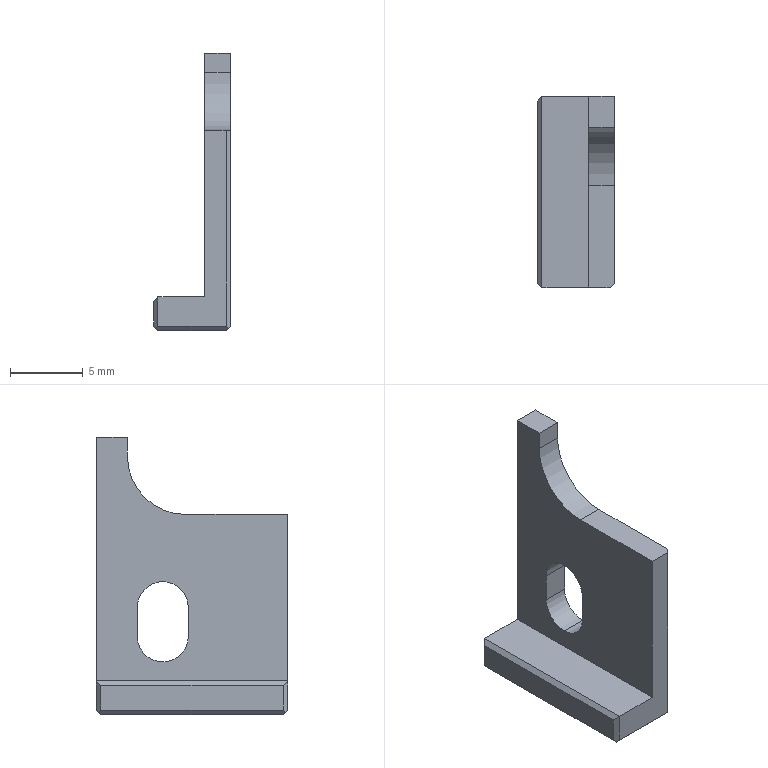Part | NX | 1 solid | 24 faces | box 5.273 x 13.1 x 19 mm | volume 417.678 mm3 | plane 20 | cylinder 4 | commonest cylinder face diameters 3.5 x3 8 x1
STEP:
#1=CARTESIAN_POINT('',(1996.107,151.5,-109.));
#2=VERTEX_POINT('',#1);
#3=CARTESIAN_POINT('',(1997.581,151.5,-109.));
#4=VERTEX_POINT('',#3);
#5=CARTESIAN_POINT('',(1996.994,151.5,-109.));
#6=DIRECTION('',(1.,0.,0.));
#7=VECTOR('',#6,1000.);
#8=LINE('',#5,#7);
#9=EDGE_CURVE('',#2,#4,#8,.T.);
#10=ORIENTED_EDGE('',*,*,#9,.F.);
#11=CARTESIAN_POINT('',(1996.107,151.5,-120.418));
#12=VERTEX_POINT('',#11);
#13=CARTESIAN_POINT('',(1996.107,151.5,-103.718));
#14=DIRECTION('',(0.,0.,-1.));
#15=VECTOR('',#14,1000.);
#16=LINE('',#13,#15);
#17=EDGE_CURVE('',#2,#12,#16,.T.);
#18=ORIENTED_EDGE('',*,*,#17,.T.);
#19=CARTESIAN_POINT('',(1992.907,151.5,-120.418));
#20=VERTEX_POINT('',#19);
#21=CARTESIAN_POINT('',(1996.107,151.5,-120.418));
#22=DIRECTION('',(-1.,0.,0.));
#23=VECTOR('',#22,1000.);
#24=LINE('',#21,#23);
#25=EDGE_CURVE('',#12,#20,#24,.T.);
#26=ORIENTED_EDGE('',*,*,#25,.T.);
#27=CARTESIAN_POINT('',(1992.907,151.5,-122.418));
#28=VERTEX_POINT('',#27);
#29=CARTESIAN_POINT('',(1992.907,151.5,-121.568));
#30=DIRECTION('',(0.,0.,-1.));
#31=VECTOR('',#30,1000.);
#32=LINE('',#29,#31);
#33=EDGE_CURVE('',#20,#28,#32,.T.);
#34=ORIENTED_EDGE('',*,*,#33,.T.);
#35=CARTESIAN_POINT('',(1997.581,151.5,-122.418));
#36=VERTEX_POINT('',#35);
#37=CARTESIAN_POINT('',(1995.244,151.5,-122.418));
#38=DIRECTION('',(-1.,0.,0.));
#39=VECTOR('',#38,1000.);
#40=LINE('',#37,#39);
#41=EDGE_CURVE('',#36,#28,#40,.T.);
#42=ORIENTED_EDGE('',*,*,#41,.F.);
#43=CARTESIAN_POINT('',(1997.581,151.5,-103.718));
#44=DIRECTION('',(0.,0.,-1.));
#45=VECTOR('',#44,1000.);
#46=LINE('',#43,#45);
#47=EDGE_CURVE('',#4,#36,#46,.T.);
#48=ORIENTED_EDGE('',*,*,#47,.F.);
#49=EDGE_LOOP('',(#10,#18,#26,#34,#42,#48));
#50=FACE_BOUND('',#49,.T.);
#51=CARTESIAN_POINT('',(1997.881,151.5,-103.718));
#52=DIRECTION('',(0.,1.,0.));
#53=DIRECTION('',(1.,0.,0.));
#54=AXIS2_PLACEMENT_3D('',#51,#52,#53);
#55=PLANE('',#54);
#56=ADVANCED_FACE('',(#50),#55,.F.);
#57=CARTESIAN_POINT('',(1997.881,151.8,-109.));
#58=VERTEX_POINT('',#57);
#59=CARTESIAN_POINT('',(1997.881,151.8,-122.418));
#60=VERTEX_POINT('',#59);
#61=CARTESIAN_POINT('',(1997.881,151.8,-115.709));
#62=DIRECTION('',(0.,0.,-1.));
#63=VECTOR('',#62,1000.);
#64=LINE('',#61,#63);
#65=EDGE_CURVE('',#58,#60,#64,.T.);
#66=ORIENTED_EDGE('',*,*,#65,.T.);
#67=CARTESIAN_POINT('',(1997.881,164.6,-122.418));
#68=VERTEX_POINT('',#67);
#69=CARTESIAN_POINT('',(1997.881,158.05,-122.418));
#70=DIRECTION('',(0.,1.,0.));
#71=VECTOR('',#70,1000.);
#72=LINE('',#69,#71);
#73=EDGE_CURVE('',#60,#68,#72,.T.);
#74=ORIENTED_EDGE('',*,*,#73,.T.);
#75=CARTESIAN_POINT('',(1997.881,164.6,-103.718));
#76=VERTEX_POINT('',#75);
#77=CARTESIAN_POINT('',(1997.881,164.6,-103.718));
#78=DIRECTION('',(0.,0.,-1.));
#79=VECTOR('',#78,1000.);
#80=LINE('',#77,#79);
#81=EDGE_CURVE('',#76,#68,#80,.T.);
#82=ORIENTED_EDGE('',*,*,#81,.F.);
#83=CARTESIAN_POINT('',(1997.881,162.476,-103.718));
#84=VERTEX_POINT('',#83);
#85=CARTESIAN_POINT('',(1997.881,155.5,-103.718));
#86=DIRECTION('',(0.,1.,0.));
#87=VECTOR('',#86,1000.);
#88=LINE('',#85,#87);
#89=EDGE_CURVE('',#84,#76,#88,.T.);
#90=ORIENTED_EDGE('',*,*,#89,.F.);
#91=CARTESIAN_POINT('',(1997.881,162.476,-105.));
#92=VERTEX_POINT('',#91);
#93=CARTESIAN_POINT('',(1997.881,162.476,-103.718));
#94=DIRECTION('',(0.,0.,1.));
#95=VECTOR('',#94,1000.);
#96=LINE('',#93,#95);
#97=EDGE_CURVE('',#92,#84,#96,.T.);
#98=ORIENTED_EDGE('',*,*,#97,.F.);
#99=CARTESIAN_POINT('',(1997.881,158.476,-109.));
#100=VERTEX_POINT('',#99);
#101=CARTESIAN_POINT('',(1997.881,158.476,-105.));
#102=DIRECTION('',(1.,0.,0.));
#103=DIRECTION('',(0.,-1.,0.));
#104=AXIS2_PLACEMENT_3D('',#101,#102,#103);
#105=CIRCLE('',#104,4.);
#106=EDGE_CURVE('',#100,#92,#105,.T.);
#107=ORIENTED_EDGE('',*,*,#106,.F.);
#108=CARTESIAN_POINT('',(1997.881,163.538,-109.));
#109=DIRECTION('',(0.,1.,0.));
#110=VECTOR('',#109,1000.);
#111=LINE('',#108,#110);
#112=EDGE_CURVE('',#58,#100,#111,.T.);
#113=ORIENTED_EDGE('',*,*,#112,.F.);
#114=EDGE_LOOP('',(#66,#74,#82,#90,#98,#107,#113));
#115=FACE_BOUND('',#114,.T.);
#116=CARTESIAN_POINT('',(1997.881,158.3,-117.359));
#117=VERTEX_POINT('',#116);
#118=CARTESIAN_POINT('',(1997.881,158.3,-115.359));
#119=VERTEX_POINT('',#118);
#120=CARTESIAN_POINT('',(1997.881,158.3,-103.718));
#121=DIRECTION('',(0.,0.,1.));
#122=VECTOR('',#121,1000.);
#123=LINE('',#120,#122);
#124=EDGE_CURVE('',#117,#119,#123,.T.);
#125=ORIENTED_EDGE('',*,*,#124,.T.);
#126=CARTESIAN_POINT('',(1997.881,161.8,-115.359));
#127=VERTEX_POINT('',#126);
#128=CARTESIAN_POINT('',(1997.881,160.05,-115.359));
#129=DIRECTION('',(1.,0.,0.));
#130=DIRECTION('',(0.,0.,-1.));
#131=AXIS2_PLACEMENT_3D('',#128,#129,#130);
#132=CIRCLE('',#131,1.75);
#133=EDGE_CURVE('',#127,#119,#132,.T.);
#134=ORIENTED_EDGE('',*,*,#133,.F.);
#135=CARTESIAN_POINT('',(1997.881,161.8,-117.359));
#136=VERTEX_POINT('',#135);
#137=CARTESIAN_POINT('',(1997.881,161.8,-103.718));
#138=DIRECTION('',(0.,0.,-1.));
#139=VECTOR('',#138,1000.);
#140=LINE('',#137,#139);
#141=EDGE_CURVE('',#127,#136,#140,.T.);
#142=ORIENTED_EDGE('',*,*,#141,.T.);
#143=CARTESIAN_POINT('',(1997.881,160.05,-119.109));
#144=VERTEX_POINT('',#143);
#145=CARTESIAN_POINT('',(1997.881,160.05,-117.359));
#146=DIRECTION('',(1.,0.,0.));
#147=DIRECTION('',(0.,0.,-1.));
#148=AXIS2_PLACEMENT_3D('',#145,#146,#147);
#149=CIRCLE('',#148,1.75);
#150=EDGE_CURVE('',#144,#136,#149,.T.);
#151=ORIENTED_EDGE('',*,*,#150,.F.);
#152=CARTESIAN_POINT('',(1997.881,160.05,-117.359));
#153=DIRECTION('',(1.,0.,0.));
#154=DIRECTION('',(0.,0.,-1.));
#155=AXIS2_PLACEMENT_3D('',#152,#153,#154);
#156=CIRCLE('',#155,1.75);
#157=EDGE_CURVE('',#117,#144,#156,.T.);
#158=ORIENTED_EDGE('',*,*,#157,.F.);
#159=EDGE_LOOP('',(#125,#134,#142,#151,#158));
#160=FACE_BOUND('',#159,.T.);
#161=CARTESIAN_POINT('',(1997.881,164.6,-103.718));
#162=DIRECTION('',(-1.,0.,0.));
#163=DIRECTION('',(0.,0.,1.));
#164=AXIS2_PLACEMENT_3D('',#161,#162,#163);
#165=PLANE('',#164);
#166=ADVANCED_FACE('',(#115,#160),#165,.F.);
#167=CARTESIAN_POINT('',(1996.107,158.476,-109.));
#168=VERTEX_POINT('',#167);
#169=CARTESIAN_POINT('',(1996.107,163.538,-109.));
#170=DIRECTION('',(0.,-1.,0.));
#171=VECTOR('',#170,1000.);
#172=LINE('',#169,#171);
#173=EDGE_CURVE('',#168,#2,#172,.T.);
#174=ORIENTED_EDGE('',*,*,#173,.F.);
#175=CARTESIAN_POINT('',(1996.107,162.476,-105.));
#176=VERTEX_POINT('',#175);
#177=CARTESIAN_POINT('',(1996.107,158.476,-105.));
#178=DIRECTION('',(1.,0.,0.));
#179=DIRECTION('',(0.,-1.,0.));
#180=AXIS2_PLACEMENT_3D('',#177,#178,#179);
#181=CIRCLE('',#180,4.);
#182=EDGE_CURVE('',#168,#176,#181,.T.);
#183=ORIENTED_EDGE('',*,*,#182,.T.);
#184=CARTESIAN_POINT('',(1996.107,162.476,-103.718));
#185=VERTEX_POINT('',#184);
#186=CARTESIAN_POINT('',(1996.107,162.476,-103.718));
#187=DIRECTION('',(0.,0.,-1.));
#188=VECTOR('',#187,1000.);
#189=LINE('',#186,#188);
#190=EDGE_CURVE('',#185,#176,#189,.T.);
#191=ORIENTED_EDGE('',*,*,#190,.F.);
#192=CARTESIAN_POINT('',(1996.107,164.6,-103.718));
#193=VERTEX_POINT('',#192);
#194=CARTESIAN_POINT('',(1996.107,164.6,-103.718));
#195=DIRECTION('',(0.,-1.,0.));
#196=VECTOR('',#195,1000.);
#197=LINE('',#194,#196);
#198=EDGE_CURVE('',#193,#185,#197,.T.);
#199=ORIENTED_EDGE('',*,*,#198,.F.);
#200=CARTESIAN_POINT('',(1996.107,164.6,-120.418));
#201=VERTEX_POINT('',#200);
#202=CARTESIAN_POINT('',(1996.107,164.6,-103.718));
#203=DIRECTION('',(0.,0.,-1.));
#204=VECTOR('',#203,1000.);
#205=LINE('',#202,#204);
#206=EDGE_CURVE('',#193,#201,#205,.T.);
#207=ORIENTED_EDGE('',*,*,#206,.T.);
#208=CARTESIAN_POINT('',(1996.107,163.538,-120.418));
#209=DIRECTION('',(0.,-1.,0.));
#210=VECTOR('',#209,1000.);
#211=LINE('',#208,#210);
#212=EDGE_CURVE('',#201,#12,#211,.T.);
#213=ORIENTED_EDGE('',*,*,#212,.T.);
#214=ORIENTED_EDGE('',*,*,#17,.F.);
#215=EDGE_LOOP('',(#174,#183,#191,#199,#207,#213,#214));
#216=FACE_BOUND('',#215,.T.);
#217=CARTESIAN_POINT('',(1996.107,158.3,-115.359));
#218=VERTEX_POINT('',#217);
#219=CARTESIAN_POINT('',(1996.107,158.3,-117.359));
#220=VERTEX_POINT('',#219);
#221=CARTESIAN_POINT('',(1996.107,158.3,-103.718));
#222=DIRECTION('',(0.,0.,-1.));
#223=VECTOR('',#222,1000.);
#224=LINE('',#221,#223);
#225=EDGE_CURVE('',#218,#220,#224,.T.);
#226=ORIENTED_EDGE('',*,*,#225,.T.);
#227=CARTESIAN_POINT('',(1996.107,160.05,-119.109));
#228=VERTEX_POINT('',#227);
#229=CARTESIAN_POINT('',(1996.107,160.05,-117.359));
#230=DIRECTION('',(1.,0.,0.));
#231=DIRECTION('',(0.,0.,-1.));
#232=AXIS2_PLACEMENT_3D('',#229,#230,#231);
#233=CIRCLE('',#232,1.75);
#234=EDGE_CURVE('',#220,#228,#233,.T.);
#235=ORIENTED_EDGE('',*,*,#234,.T.);
#236=CARTESIAN_POINT('',(1996.107,161.8,-117.359));
#237=VERTEX_POINT('',#236);
#238=CARTESIAN_POINT('',(1996.107,160.05,-117.359));
#239=DIRECTION('',(1.,0.,0.));
#240=DIRECTION('',(0.,0.,-1.));
#241=AXIS2_PLACEMENT_3D('',#238,#239,#240);
#242=CIRCLE('',#241,1.75);
#243=EDGE_CURVE('',#228,#237,#242,.T.);
#244=ORIENTED_EDGE('',*,*,#243,.T.);
#245=CARTESIAN_POINT('',(1996.107,161.8,-115.359));
#246=VERTEX_POINT('',#245);
#247=CARTESIAN_POINT('',(1996.107,161.8,-103.718));
#248=DIRECTION('',(0.,0.,1.));
#249=VECTOR('',#248,1000.);
#250=LINE('',#247,#249);
#251=EDGE_CURVE('',#237,#246,#250,.T.);
#252=ORIENTED_EDGE('',*,*,#251,.T.);
#253=CARTESIAN_POINT('',(1996.107,160.05,-115.359));
#254=DIRECTION('',(1.,0.,0.));
#255=DIRECTION('',(0.,0.,-1.));
#256=AXIS2_PLACEMENT_3D('',#253,#254,#255);
#257=CIRCLE('',#256,1.75);
#258=EDGE_CURVE('',#246,#218,#257,.T.);
#259=ORIENTED_EDGE('',*,*,#258,.T.);
#260=EDGE_LOOP('',(#226,#235,#244,#252,#259));
#261=FACE_BOUND('',#260,.T.);
#262=CARTESIAN_POINT('',(1996.107,155.5,-103.718));
#263=DIRECTION('',(1.,0.,0.));
#264=DIRECTION('',(0.,1.,0.));
#265=AXIS2_PLACEMENT_3D('',#262,#263,#264);
#266=PLANE('',#265);
#267=ADVANCED_FACE('',(#216,#261),#266,.F.);
#268=CARTESIAN_POINT('',(1992.907,164.6,-122.418));
#269=VERTEX_POINT('',#268);
#270=CARTESIAN_POINT('',(1995.244,164.6,-122.418));
#271=DIRECTION('',(1.,0.,0.));
#272=VECTOR('',#271,1000.);
#273=LINE('',#270,#272);
#274=EDGE_CURVE('',#269,#68,#273,.T.);
#275=ORIENTED_EDGE('',*,*,#274,.F.);
#276=CARTESIAN_POINT('',(1992.907,164.6,-120.418));
#277=VERTEX_POINT('',#276);
#278=CARTESIAN_POINT('',(1992.907,164.6,-121.568));
#279=DIRECTION('',(0.,0.,1.));
#280=VECTOR('',#279,1000.);
#281=LINE('',#278,#280);
#282=EDGE_CURVE('',#269,#277,#281,.T.);
#283=ORIENTED_EDGE('',*,*,#282,.T.);
#284=CARTESIAN_POINT('',(1996.107,164.6,-120.418));
#285=DIRECTION('',(-1.,0.,0.));
#286=VECTOR('',#285,1000.);
#287=LINE('',#284,#286);
#288=EDGE_CURVE('',#201,#277,#287,.T.);
#289=ORIENTED_EDGE('',*,*,#288,.F.);
#290=ORIENTED_EDGE('',*,*,#206,.F.);
#291=CARTESIAN_POINT('',(2001.481,164.6,-103.718));
#292=DIRECTION('',(-1.,0.,0.));
#293=VECTOR('',#292,1000.);
#294=LINE('',#291,#293);
#295=EDGE_CURVE('',#76,#193,#294,.T.);
#296=ORIENTED_EDGE('',*,*,#295,.F.);
#297=ORIENTED_EDGE('',*,*,#81,.T.);
#298=EDGE_LOOP('',(#275,#283,#289,#290,#296,#297));
#299=FACE_BOUND('',#298,.T.);
#300=CARTESIAN_POINT('',(1996.107,164.6,-103.718));
#301=DIRECTION('',(0.,-1.,0.));
#302=DIRECTION('',(0.,0.,-1.));
#303=AXIS2_PLACEMENT_3D('',#300,#301,#302);
#304=PLANE('',#303);
#305=ADVANCED_FACE('',(#299),#304,.F.);
#306=CARTESIAN_POINT('',(1993.73,160.05,-119.109));
#307=DIRECTION('',(1.,0.,0.));
#308=VECTOR('',#307,1000.);
#309=LINE('',#306,#308);
#310=EDGE_CURVE('',#228,#144,#309,.T.);
#311=ORIENTED_EDGE('',*,*,#310,.F.);
#312=ORIENTED_EDGE('',*,*,#234,.F.);
#313=CARTESIAN_POINT('',(1993.73,158.3,-117.359));
#314=DIRECTION('',(1.,0.,0.));
#315=VECTOR('',#314,1000.);
#316=LINE('',#313,#315);
#317=EDGE_CURVE('',#220,#117,#316,.T.);
#318=ORIENTED_EDGE('',*,*,#317,.T.);
#319=ORIENTED_EDGE('',*,*,#157,.T.);
#320=EDGE_LOOP('',(#311,#312,#318,#319));
#321=FACE_BOUND('',#320,.T.);
#322=CARTESIAN_POINT('',(1993.73,160.05,-117.359));
#323=DIRECTION('',(1.,0.,0.));
#324=DIRECTION('',(0.,0.,-1.));
#325=AXIS2_PLACEMENT_3D('',#322,#323,#324);
#326=CYLINDRICAL_SURFACE('',#325,1.75);
#327=ADVANCED_FACE('',(#321),#326,.F.);
#328=ORIENTED_EDGE('',*,*,#251,.F.);
#329=CARTESIAN_POINT('',(1993.73,161.8,-117.359));
#330=DIRECTION('',(1.,0.,0.));
#331=VECTOR('',#330,1000.);
#332=LINE('',#329,#331);
#333=EDGE_CURVE('',#237,#136,#332,.T.);
#334=ORIENTED_EDGE('',*,*,#333,.T.);
#335=ORIENTED_EDGE('',*,*,#141,.F.);
#336=CARTESIAN_POINT('',(1993.73,161.8,-115.359));
#337=DIRECTION('',(1.,0.,0.));
#338=VECTOR('',#337,1000.);
#339=LINE('',#336,#338);
#340=EDGE_CURVE('',#246,#127,#339,.T.);
#341=ORIENTED_EDGE('',*,*,#340,.F.);
#342=EDGE_LOOP('',(#328,#334,#335,#341));
#343=FACE_BOUND('',#342,.T.);
#344=CARTESIAN_POINT('',(1993.73,161.8,-115.359));
#345=DIRECTION('',(0.,1.,0.));
#346=DIRECTION('',(1.,0.,0.));
#347=AXIS2_PLACEMENT_3D('',#344,#345,#346);
#348=PLANE('',#347);
#349=ADVANCED_FACE('',(#343),#348,.F.);
#350=ORIENTED_EDGE('',*,*,#258,.F.);
#351=ORIENTED_EDGE('',*,*,#340,.T.);
#352=ORIENTED_EDGE('',*,*,#133,.T.);
#353=CARTESIAN_POINT('',(1993.73,158.3,-115.359));
#354=DIRECTION('',(1.,0.,0.));
#355=VECTOR('',#354,1000.);
#356=LINE('',#353,#355);
#357=EDGE_CURVE('',#218,#119,#356,.T.);
#358=ORIENTED_EDGE('',*,*,#357,.F.);
#359=EDGE_LOOP('',(#350,#351,#352,#358));
#360=FACE_BOUND('',#359,.T.);
#361=CARTESIAN_POINT('',(1993.73,160.05,-115.359));
#362=DIRECTION('',(1.,0.,0.));
#363=DIRECTION('',(0.,0.,-1.));
#364=AXIS2_PLACEMENT_3D('',#361,#362,#363);
#365=CYLINDRICAL_SURFACE('',#364,1.75);
#366=ADVANCED_FACE('',(#360),#365,.F.);
#367=ORIENTED_EDGE('',*,*,#225,.F.);
#368=ORIENTED_EDGE('',*,*,#357,.T.);
#369=ORIENTED_EDGE('',*,*,#124,.F.);
#370=ORIENTED_EDGE('',*,*,#317,.F.);
#371=EDGE_LOOP('',(#367,#368,#369,#370));
#372=FACE_BOUND('',#371,.T.);
#373=CARTESIAN_POINT('',(1993.73,158.3,-117.359));
#374=DIRECTION('',(0.,-1.,0.));
#375=DIRECTION('',(0.,0.,-1.));
#376=AXIS2_PLACEMENT_3D('',#373,#374,#375);
#377=PLANE('',#376);
#378=ADVANCED_FACE('',(#372),#377,.F.);
#379=ORIENTED_EDGE('',*,*,#47,.T.);
#380=CARTESIAN_POINT('',(1997.731,151.65,-122.568));
#381=VERTEX_POINT('',#380);
#382=CARTESIAN_POINT('',(2009.619,163.538,-134.456));
#383=DIRECTION('',(0.5774,0.5774,-0.5774));
#384=VECTOR('',#383,1000.);
#385=LINE('',#382,#384);
#386=EDGE_CURVE('',#36,#381,#385,.T.);
#387=ORIENTED_EDGE('',*,*,#386,.T.);
#388=CARTESIAN_POINT('',(2016.581,170.5,-103.718));
#389=DIRECTION('',(-0.5774,-0.5774,-0.5774));
#390=VECTOR('',#389,1000.);
#391=LINE('',#388,#390);
#392=EDGE_CURVE('',#60,#381,#391,.T.);
#393=ORIENTED_EDGE('',*,*,#392,.F.);
#394=ORIENTED_EDGE('',*,*,#65,.F.);
#395=CARTESIAN_POINT('',(2009.619,163.538,-109.));
#396=DIRECTION('',(-0.7071,-0.7071,0.));
#397=VECTOR('',#396,1000.);
#398=LINE('',#395,#397);
#399=EDGE_CURVE('',#58,#4,#398,.T.);
#400=ORIENTED_EDGE('',*,*,#399,.T.);
#401=EDGE_LOOP('',(#379,#387,#393,#394,#400));
#402=FACE_BOUND('',#401,.T.);
#403=CARTESIAN_POINT('',(1997.731,151.65,-115.709));
#404=DIRECTION('',(0.7071,-0.7071,0.));
#405=DIRECTION('',(0.,0.,-1.));
#406=AXIS2_PLACEMENT_3D('',#403,#404,#405);
#407=PLANE('',#406);
#408=ADVANCED_FACE('',(#402),#407,.T.);
#409=CARTESIAN_POINT('',(1996.994,158.476,-109.));
#410=DIRECTION('',(1.,0.,0.));
#411=VECTOR('',#410,1000.);
#412=LINE('',#409,#411);
#413=EDGE_CURVE('',#168,#100,#412,.T.);
#414=ORIENTED_EDGE('',*,*,#413,.T.);
#415=ORIENTED_EDGE('',*,*,#106,.T.);
#416=CARTESIAN_POINT('',(1996.994,162.476,-105.));
#417=DIRECTION('',(1.,0.,0.));
#418=VECTOR('',#417,1000.);
#419=LINE('',#416,#418);
#420=EDGE_CURVE('',#176,#92,#419,.T.);
#421=ORIENTED_EDGE('',*,*,#420,.F.);
#422=ORIENTED_EDGE('',*,*,#182,.F.);
#423=EDGE_LOOP('',(#414,#415,#421,#422));
#424=FACE_BOUND('',#423,.T.);
#425=CARTESIAN_POINT('',(1996.994,158.476,-105.));
#426=DIRECTION('',(1.,0.,0.));
#427=DIRECTION('',(0.,-1.,0.));
#428=AXIS2_PLACEMENT_3D('',#425,#426,#427);
#429=CYLINDRICAL_SURFACE('',#428,4.);
#430=ADVANCED_FACE('',(#424),#429,.F.);
#431=ORIENTED_EDGE('',*,*,#212,.F.);
#432=ORIENTED_EDGE('',*,*,#288,.T.);
#433=CARTESIAN_POINT('',(1992.907,158.05,-120.418));
#434=DIRECTION('',(0.,-1.,0.));
#435=VECTOR('',#434,1000.);
#436=LINE('',#433,#435);
#437=EDGE_CURVE('',#277,#20,#436,.T.);
#438=ORIENTED_EDGE('',*,*,#437,.T.);
#439=ORIENTED_EDGE('',*,*,#25,.F.);
#440=EDGE_LOOP('',(#431,#432,#438,#439));
#441=FACE_BOUND('',#440,.T.);
#442=CARTESIAN_POINT('',(1996.107,164.6,-120.418));
#443=DIRECTION('',(0.,0.,1.));
#444=DIRECTION('',(1.,0.,0.));
#445=AXIS2_PLACEMENT_3D('',#442,#443,#444);
#446=PLANE('',#445);
#447=ADVANCED_FACE('',(#441),#446,.T.);
#448=CARTESIAN_POINT('',(1992.607,164.3,-122.418));
#449=VERTEX_POINT('',#448);
#450=CARTESIAN_POINT('',(1992.607,164.3,-120.718));
#451=VERTEX_POINT('',#450);
#452=CARTESIAN_POINT('',(1992.607,164.3,-121.568));
#453=DIRECTION('',(0.,0.,1.));
#454=VECTOR('',#453,1000.);
#455=LINE('',#452,#454);
#456=EDGE_CURVE('',#449,#451,#455,.T.);
#457=ORIENTED_EDGE('',*,*,#456,.F.);
#458=CARTESIAN_POINT('',(1992.607,151.8,-122.418));
#459=VERTEX_POINT('',#458);
#460=CARTESIAN_POINT('',(1992.607,158.05,-122.418));
#461=DIRECTION('',(0.,-1.,0.));
#462=VECTOR('',#461,1000.);
#463=LINE('',#460,#462);
#464=EDGE_CURVE('',#449,#459,#463,.T.);
#465=ORIENTED_EDGE('',*,*,#464,.T.);
#466=CARTESIAN_POINT('',(1992.607,151.8,-120.718));
#467=VERTEX_POINT('',#466);
#468=CARTESIAN_POINT('',(1992.607,151.8,-121.568));
#469=DIRECTION('',(0.,0.,-1.));
#470=VECTOR('',#469,1000.);
#471=LINE('',#468,#470);
#472=EDGE_CURVE('',#467,#459,#471,.T.);
#473=ORIENTED_EDGE('',*,*,#472,.F.);
#474=CARTESIAN_POINT('',(1992.607,158.05,-120.718));
#475=DIRECTION('',(0.,-1.,0.));
#476=VECTOR('',#475,1000.);
#477=LINE('',#474,#476);
#478=EDGE_CURVE('',#451,#467,#477,.T.);
#479=ORIENTED_EDGE('',*,*,#478,.F.);
#480=EDGE_LOOP('',(#457,#465,#473,#479));
#481=FACE_BOUND('',#480,.T.);
#482=CARTESIAN_POINT('',(1992.607,160.05,-113.718));
#483=DIRECTION('',(-1.,0.,0.));
#484=DIRECTION('',(0.,0.,1.));
#485=AXIS2_PLACEMENT_3D('',#482,#483,#484);
#486=PLANE('',#485);
#487=ADVANCED_FACE('',(#481),#486,.T.);
#488=CARTESIAN_POINT('',(1996.994,162.476,-103.718));
#489=DIRECTION('',(1.,0.,0.));
#490=VECTOR('',#489,1000.);
#491=LINE('',#488,#490);
#492=EDGE_CURVE('',#185,#84,#491,.T.);
#493=ORIENTED_EDGE('',*,*,#492,.F.);
#494=ORIENTED_EDGE('',*,*,#190,.T.);
#495=ORIENTED_EDGE('',*,*,#420,.T.);
#496=ORIENTED_EDGE('',*,*,#97,.T.);
#497=EDGE_LOOP('',(#493,#494,#495,#496));
#498=FACE_BOUND('',#497,.T.);
#499=CARTESIAN_POINT('',(1996.107,162.476,-103.718));
#500=DIRECTION('',(0.,-1.,0.));
#501=DIRECTION('',(0.,0.,-1.));
#502=AXIS2_PLACEMENT_3D('',#499,#500,#501);
#503=PLANE('',#502);
#504=ADVANCED_FACE('',(#498),#503,.T.);
#505=ORIENTED_EDGE('',*,*,#399,.F.);
#506=ORIENTED_EDGE('',*,*,#112,.T.);
#507=ORIENTED_EDGE('',*,*,#413,.F.);
#508=ORIENTED_EDGE('',*,*,#173,.T.);
#509=ORIENTED_EDGE('',*,*,#9,.T.);
#510=EDGE_LOOP('',(#505,#506,#507,#508,#509));
#511=FACE_BOUND('',#510,.T.);
#512=CARTESIAN_POINT('',(1996.994,163.538,-109.));
#513=DIRECTION('',(0.,0.,1.));
#514=DIRECTION('',(1.,0.,0.));
#515=AXIS2_PLACEMENT_3D('',#512,#513,#514);
#516=PLANE('',#515);
#517=ADVANCED_FACE('',(#511),#516,.T.);
#518=ORIENTED_EDGE('',*,*,#472,.T.);
#519=CARTESIAN_POINT('',(1992.757,151.65,-122.568));
#520=VERTEX_POINT('',#519);
#521=CARTESIAN_POINT('',(1973.907,170.5,-103.718));
#522=DIRECTION('',(-0.5774,0.5774,0.5774));
#523=VECTOR('',#522,1000.);
#524=LINE('',#521,#523);
#525=EDGE_CURVE('',#520,#459,#524,.T.);
#526=ORIENTED_EDGE('',*,*,#525,.F.);
#527=CARTESIAN_POINT('',(2011.607,132.8,-103.718));
#528=DIRECTION('',(0.5774,-0.5774,0.5774));
#529=VECTOR('',#528,1000.);
#530=LINE('',#527,#529);
#531=EDGE_CURVE('',#520,#28,#530,.T.);
#532=ORIENTED_EDGE('',*,*,#531,.T.);
#533=ORIENTED_EDGE('',*,*,#33,.F.);
#534=CARTESIAN_POINT('',(2009.607,134.8,-103.718));
#535=DIRECTION('',(-0.5774,0.5774,-0.5774));
#536=VECTOR('',#535,1000.);
#537=LINE('',#534,#536);
#538=EDGE_CURVE('',#20,#467,#537,.T.);
#539=ORIENTED_EDGE('',*,*,#538,.T.);
#540=EDGE_LOOP('',(#518,#526,#532,#533,#539));
#541=FACE_BOUND('',#540,.T.);
#542=CARTESIAN_POINT('',(1992.757,151.65,-121.568));
#543=DIRECTION('',(0.7071,0.7071,0.));
#544=DIRECTION('',(0.,0.,-1.));
#545=AXIS2_PLACEMENT_3D('',#542,#543,#544);
#546=PLANE('',#545);
#547=ADVANCED_FACE('',(#541),#546,.F.);
#548=ORIENTED_EDGE('',*,*,#478,.T.);
#549=ORIENTED_EDGE('',*,*,#538,.F.);
#550=ORIENTED_EDGE('',*,*,#437,.F.);
#551=CARTESIAN_POINT('',(2009.607,181.3,-103.718));
#552=DIRECTION('',(-0.5774,-0.5774,-0.5774));
#553=VECTOR('',#552,1000.);
#554=LINE('',#551,#553);
#555=EDGE_CURVE('',#277,#451,#554,.T.);
#556=ORIENTED_EDGE('',*,*,#555,.T.);
#557=EDGE_LOOP('',(#548,#549,#550,#556));
#558=FACE_BOUND('',#557,.T.);
#559=CARTESIAN_POINT('',(1992.757,158.05,-120.568));
#560=DIRECTION('',(0.7071,0.,-0.7071));
#561=DIRECTION('',(0.,-1.,0.));
#562=AXIS2_PLACEMENT_3D('',#559,#560,#561);
#563=PLANE('',#562);
#564=ADVANCED_FACE('',(#558),#563,.F.);
#565=ORIENTED_EDGE('',*,*,#456,.T.);
#566=ORIENTED_EDGE('',*,*,#555,.F.);
#567=ORIENTED_EDGE('',*,*,#282,.F.);
#568=CARTESIAN_POINT('',(1992.757,164.45,-122.568));
#569=VERTEX_POINT('',#568);
#570=CARTESIAN_POINT('',(2011.607,183.3,-103.718));
#571=DIRECTION('',(-0.5774,-0.5774,-0.5774));
#572=VECTOR('',#571,1000.);
#573=LINE('',#570,#572);
#574=EDGE_CURVE('',#269,#569,#573,.T.);
#575=ORIENTED_EDGE('',*,*,#574,.T.);
#576=CARTESIAN_POINT('',(1973.907,145.6,-103.718));
#577=DIRECTION('',(0.5774,0.5774,-0.5774));
#578=VECTOR('',#577,1000.);
#579=LINE('',#576,#578);
#580=EDGE_CURVE('',#449,#569,#579,.T.);
#581=ORIENTED_EDGE('',*,*,#580,.F.);
#582=EDGE_LOOP('',(#565,#566,#567,#575,#581));
#583=FACE_BOUND('',#582,.T.);
#584=CARTESIAN_POINT('',(1992.757,164.45,-121.568));
#585=DIRECTION('',(0.7071,-0.7071,0.));
#586=DIRECTION('',(0.,0.,-1.));
#587=AXIS2_PLACEMENT_3D('',#584,#585,#586);
#588=PLANE('',#587);
#589=ADVANCED_FACE('',(#583),#588,.F.);
#590=CARTESIAN_POINT('',(1997.581,151.8,-122.718));
#591=VERTEX_POINT('',#590);
#592=CARTESIAN_POINT('',(1992.907,151.8,-122.718));
#593=VERTEX_POINT('',#592);
#594=CARTESIAN_POINT('',(1995.244,151.8,-122.718));
#595=DIRECTION('',(-1.,0.,0.));
#596=VECTOR('',#595,1000.);
#597=LINE('',#594,#596);
#598=EDGE_CURVE('',#591,#593,#597,.T.);
#599=ORIENTED_EDGE('',*,*,#598,.T.);
#600=CARTESIAN_POINT('',(1992.907,164.3,-122.718));
#601=VERTEX_POINT('',#600);
#602=CARTESIAN_POINT('',(1992.907,158.05,-122.718));
#603=DIRECTION('',(0.,-1.,0.));
#604=VECTOR('',#603,1000.);
#605=LINE('',#602,#604);
#606=EDGE_CURVE('',#601,#593,#605,.T.);
#607=ORIENTED_EDGE('',*,*,#606,.F.);
#608=CARTESIAN_POINT('',(1997.581,164.3,-122.718));
#609=VERTEX_POINT('',#608);
#610=CARTESIAN_POINT('',(1995.244,164.3,-122.718));
#611=DIRECTION('',(1.,0.,0.));
#612=VECTOR('',#611,1000.);
#613=LINE('',#610,#612);
#614=EDGE_CURVE('',#601,#609,#613,.T.);
#615=ORIENTED_EDGE('',*,*,#614,.T.);
#616=CARTESIAN_POINT('',(1997.581,158.05,-122.718));
#617=DIRECTION('',(0.,1.,0.));
#618=VECTOR('',#617,1000.);
#619=LINE('',#616,#618);
#620=EDGE_CURVE('',#591,#609,#619,.T.);
#621=ORIENTED_EDGE('',*,*,#620,.F.);
#622=EDGE_LOOP('',(#599,#607,#615,#621));
#623=FACE_BOUND('',#622,.T.);
#624=CARTESIAN_POINT('',(1996.994,163.538,-122.718));
#625=DIRECTION('',(0.,0.,1.));
#626=DIRECTION('',(1.,0.,0.));
#627=AXIS2_PLACEMENT_3D('',#624,#625,#626);
#628=PLANE('',#627);
#629=ADVANCED_FACE('',(#623),#628,.F.);
#630=ORIENTED_EDGE('',*,*,#620,.T.);
#631=CARTESIAN_POINT('',(2016.581,183.3,-103.718));
#632=DIRECTION('',(-0.5774,-0.5774,-0.5774));
#633=VECTOR('',#632,1000.);
#634=LINE('',#631,#633);
#635=EDGE_CURVE('',#68,#609,#634,.T.);
#636=ORIENTED_EDGE('',*,*,#635,.F.);
#637=ORIENTED_EDGE('',*,*,#73,.F.);
#638=ORIENTED_EDGE('',*,*,#392,.T.);
#639=CARTESIAN_POINT('',(2016.581,132.8,-103.718));
#640=DIRECTION('',(0.5774,-0.5774,0.5774));
#641=VECTOR('',#640,1000.);
#642=LINE('',#639,#641);
#643=EDGE_CURVE('',#591,#381,#642,.T.);
#644=ORIENTED_EDGE('',*,*,#643,.F.);
#645=EDGE_LOOP('',(#630,#636,#637,#638,#644));
#646=FACE_BOUND('',#645,.T.);
#647=CARTESIAN_POINT('',(1997.731,158.05,-122.568));
#648=DIRECTION('',(-0.7071,0.,0.7071));
#649=DIRECTION('',(0.,1.,0.));
#650=AXIS2_PLACEMENT_3D('',#647,#648,#649);
#651=PLANE('',#650);
#652=ADVANCED_FACE('',(#646),#651,.F.);
#653=ORIENTED_EDGE('',*,*,#606,.T.);
#654=CARTESIAN_POINT('',(1973.907,132.8,-103.718));
#655=DIRECTION('',(0.5774,0.5774,-0.5774));
#656=VECTOR('',#655,1000.);
#657=LINE('',#654,#656);
#658=EDGE_CURVE('',#520,#593,#657,.T.);
#659=ORIENTED_EDGE('',*,*,#658,.F.);
#660=ORIENTED_EDGE('',*,*,#525,.T.);
#661=ORIENTED_EDGE('',*,*,#464,.F.);
#662=ORIENTED_EDGE('',*,*,#580,.T.);
#663=CARTESIAN_POINT('',(1973.907,183.3,-103.718));
#664=DIRECTION('',(-0.5774,0.5774,0.5774));
#665=VECTOR('',#664,1000.);
#666=LINE('',#663,#665);
#667=EDGE_CURVE('',#601,#569,#666,.T.);
#668=ORIENTED_EDGE('',*,*,#667,.F.);
#669=EDGE_LOOP('',(#653,#659,#660,#661,#662,#668));
#670=FACE_BOUND('',#669,.T.);
#671=CARTESIAN_POINT('',(1992.757,158.05,-122.568));
#672=DIRECTION('',(0.7071,0.,0.7071));
#673=DIRECTION('',(0.,-1.,0.));
#674=AXIS2_PLACEMENT_3D('',#671,#672,#673);
#675=PLANE('',#674);
#676=ADVANCED_FACE('',(#670),#675,.F.);
#677=ORIENTED_EDGE('',*,*,#614,.F.);
#678=ORIENTED_EDGE('',*,*,#667,.T.);
#679=ORIENTED_EDGE('',*,*,#574,.F.);
#680=ORIENTED_EDGE('',*,*,#274,.T.);
#681=ORIENTED_EDGE('',*,*,#635,.T.);
#682=EDGE_LOOP('',(#677,#678,#679,#680,#681));
#683=FACE_BOUND('',#682,.T.);
#684=CARTESIAN_POINT('',(1995.244,164.45,-122.568));
#685=DIRECTION('',(0.,0.7071,-0.7071));
#686=DIRECTION('',(-1.,0.,0.));
#687=AXIS2_PLACEMENT_3D('',#684,#685,#686);
#688=PLANE('',#687);
#689=ADVANCED_FACE('',(#683),#688,.T.);
#690=ORIENTED_EDGE('',*,*,#598,.F.);
#691=ORIENTED_EDGE('',*,*,#643,.T.);
#692=ORIENTED_EDGE('',*,*,#386,.F.);
#693=ORIENTED_EDGE('',*,*,#41,.T.);
#694=ORIENTED_EDGE('',*,*,#531,.F.);
#695=ORIENTED_EDGE('',*,*,#658,.T.);
#696=EDGE_LOOP('',(#690,#691,#692,#693,#694,#695));
#697=FACE_BOUND('',#696,.T.);
#698=CARTESIAN_POINT('',(1995.244,151.65,-122.568));
#699=DIRECTION('',(0.,-0.7071,-0.7071));
#700=DIRECTION('',(0.,-0.7071,0.7071));
#701=AXIS2_PLACEMENT_3D('',#698,#699,#700);
#702=PLANE('',#701);
#703=ADVANCED_FACE('',(#697),#702,.T.);
#704=ORIENTED_EDGE('',*,*,#89,.T.);
#705=ORIENTED_EDGE('',*,*,#295,.T.);
#706=ORIENTED_EDGE('',*,*,#198,.T.);
#707=ORIENTED_EDGE('',*,*,#492,.T.);
#708=EDGE_LOOP('',(#704,#705,#706,#707));
#709=FACE_BOUND('',#708,.T.);
#710=CARTESIAN_POINT('',(1996.994,163.538,-103.718));
#711=DIRECTION('',(0.,0.,1.));
#712=DIRECTION('',(1.,0.,0.));
#713=AXIS2_PLACEMENT_3D('',#710,#711,#712);
#714=PLANE('',#713);
#715=ADVANCED_FACE('',(#709),#714,.T.);
#716=ORIENTED_EDGE('',*,*,#243,.F.);
#717=ORIENTED_EDGE('',*,*,#310,.T.);
#718=ORIENTED_EDGE('',*,*,#150,.T.);
#719=ORIENTED_EDGE('',*,*,#333,.F.);
#720=EDGE_LOOP('',(#716,#717,#718,#719));
#721=FACE_BOUND('',#720,.T.);
#722=CARTESIAN_POINT('',(1993.73,160.05,-117.359));
#723=DIRECTION('',(1.,0.,0.));
#724=DIRECTION('',(0.,0.,-1.));
#725=AXIS2_PLACEMENT_3D('',#722,#723,#724);
#726=CYLINDRICAL_SURFACE('',#725,1.75);
#727=ADVANCED_FACE('',(#721),#726,.F.);
#728=CLOSED_SHELL('',(#56,#166,#267,#305,#327,#349,#366,#378,#408,#430,#447,#487,#504,#517,#547,#564,#589,#629,#652,#676,#689,#703,#715,#727));
#729=MANIFOLD_SOLID_BREP('',#728);
#730=(LENGTH_UNIT()NAMED_UNIT(*)SI_UNIT(.MILLI.,.METRE.));
#731=UNCERTAINTY_MEASURE_WITH_UNIT(LENGTH_MEASURE(0.00001),#730,'','');
#732=(NAMED_UNIT(*)PLANE_ANGLE_UNIT()SI_UNIT($,.RADIAN.));
#733=(NAMED_UNIT(*)SI_UNIT($,.STERADIAN.)SOLID_ANGLE_UNIT());
#734=(GEOMETRIC_REPRESENTATION_CONTEXT(3)GLOBAL_UNCERTAINTY_ASSIGNED_CONTEXT((#731))GLOBAL_UNIT_ASSIGNED_CONTEXT((#730,#732,#733))REPRESENTATION_CONTEXT('',''));
#735=ADVANCED_BREP_SHAPE_REPRESENTATION('',(#729),#734);